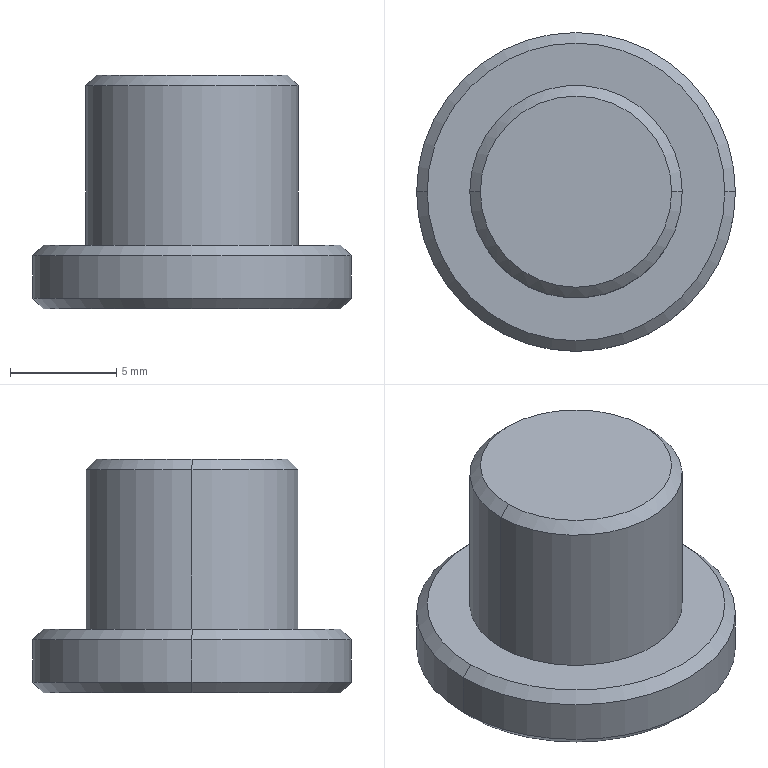Part | SolidWorks | features Chamfer 1, Revolution 1 | 1 solid | 13 faces | box 15 x 15 x 11 mm | volume 1143 mm3 | cone 6 | cylinder 4 | plane 3 | commonest cylinder face diameters 10 x2 15 x2
STEP:
#1=CARTESIAN_POINT('',(4.5,0.,0.));
#2=VERTEX_POINT('',#1);
#3=CARTESIAN_POINT('',(-4.5,0.,0.));
#4=VERTEX_POINT('',#3);
#5=CARTESIAN_POINT('',(0.,0.,0.));
#6=DIRECTION('',(0.,0.,1.));
#7=DIRECTION('',(-1.,0.,0.));
#8=AXIS2_PLACEMENT_3D('',#5,#6,#7);
#9=CIRCLE('',#8,4.5);
#10=EDGE_CURVE('',#2,#4,#9,.T.);
#11=ORIENTED_EDGE('',*,*,#10,.F.);
#12=CARTESIAN_POINT('',(5.,0.,-0.5));
#13=VERTEX_POINT('',#12);
#14=CARTESIAN_POINT('',(4.5,0.,0.));
#15=DIRECTION('',(0.7071,0.,-0.7071));
#16=VECTOR('',#15,1000.);
#17=LINE('',#14,#16);
#18=EDGE_CURVE('',#2,#13,#17,.T.);
#19=ORIENTED_EDGE('',*,*,#18,.T.);
#20=CARTESIAN_POINT('',(-5.,0.,-0.5));
#21=VERTEX_POINT('',#20);
#22=CARTESIAN_POINT('',(0.,0.,-0.5));
#23=DIRECTION('',(0.,0.,-1.));
#24=DIRECTION('',(-1.,0.,0.));
#25=AXIS2_PLACEMENT_3D('',#22,#23,#24);
#26=CIRCLE('',#25,5.);
#27=EDGE_CURVE('',#21,#13,#26,.T.);
#28=ORIENTED_EDGE('',*,*,#27,.F.);
#29=CARTESIAN_POINT('',(-4.5,0.,0.));
#30=DIRECTION('',(-0.7071,0.,-0.7071));
#31=VECTOR('',#30,1000.);
#32=LINE('',#29,#31);
#33=EDGE_CURVE('',#4,#21,#32,.T.);
#34=ORIENTED_EDGE('',*,*,#33,.F.);
#35=EDGE_LOOP('',(#11,#19,#28,#34));
#36=FACE_OUTER_BOUND('',#35,.T.);
#37=CARTESIAN_POINT('',(0.,0.,0.));
#38=DIRECTION('',(0.,0.,-1.));
#39=DIRECTION('',(-1.,0.,0.));
#40=AXIS2_PLACEMENT_3D('',#37,#38,#39);
#41=CONICAL_SURFACE('',#40,4.5,0.7854);
#42=ADVANCED_FACE('',(#36),#41,.T.);
#43=CARTESIAN_POINT('',(7.,0.,-8.));
#44=VERTEX_POINT('',#43);
#45=CARTESIAN_POINT('',(-7.,0.,-8.));
#46=VERTEX_POINT('',#45);
#47=CARTESIAN_POINT('',(0.,0.,-8.));
#48=DIRECTION('',(0.,0.,1.));
#49=DIRECTION('',(-1.,0.,0.));
#50=AXIS2_PLACEMENT_3D('',#47,#48,#49);
#51=CIRCLE('',#50,7.);
#52=EDGE_CURVE('',#44,#46,#51,.T.);
#53=ORIENTED_EDGE('',*,*,#52,.F.);
#54=CARTESIAN_POINT('',(7.5,0.,-8.5));
#55=VERTEX_POINT('',#54);
#56=CARTESIAN_POINT('',(7.,0.,-8.));
#57=DIRECTION('',(0.7071,0.,-0.7071));
#58=VECTOR('',#57,1000.);
#59=LINE('',#56,#58);
#60=EDGE_CURVE('',#44,#55,#59,.T.);
#61=ORIENTED_EDGE('',*,*,#60,.T.);
#62=CARTESIAN_POINT('',(-7.5,0.,-8.5));
#63=VERTEX_POINT('',#62);
#64=CARTESIAN_POINT('',(0.,0.,-8.5));
#65=DIRECTION('',(0.,0.,-1.));
#66=DIRECTION('',(-1.,0.,0.));
#67=AXIS2_PLACEMENT_3D('',#64,#65,#66);
#68=CIRCLE('',#67,7.5);
#69=EDGE_CURVE('',#63,#55,#68,.T.);
#70=ORIENTED_EDGE('',*,*,#69,.F.);
#71=CARTESIAN_POINT('',(-7.,0.,-8.));
#72=DIRECTION('',(-0.7071,0.,-0.7071));
#73=VECTOR('',#72,1000.);
#74=LINE('',#71,#73);
#75=EDGE_CURVE('',#46,#63,#74,.T.);
#76=ORIENTED_EDGE('',*,*,#75,.F.);
#77=EDGE_LOOP('',(#53,#61,#70,#76));
#78=FACE_OUTER_BOUND('',#77,.T.);
#79=CARTESIAN_POINT('',(0.,0.,-8.));
#80=DIRECTION('',(0.,0.,-1.));
#81=DIRECTION('',(-1.,0.,0.));
#82=AXIS2_PLACEMENT_3D('',#79,#80,#81);
#83=CONICAL_SURFACE('',#82,7.,0.7854);
#84=ADVANCED_FACE('',(#78),#83,.T.);
#85=CARTESIAN_POINT('',(-7.,0.,-11.));
#86=VERTEX_POINT('',#85);
#87=CARTESIAN_POINT('',(7.,0.,-11.));
#88=VERTEX_POINT('',#87);
#89=CARTESIAN_POINT('',(0.,0.,-11.));
#90=DIRECTION('',(0.,0.,-1.));
#91=DIRECTION('',(1.,0.,0.));
#92=AXIS2_PLACEMENT_3D('',#89,#90,#91);
#93=CIRCLE('',#92,7.);
#94=EDGE_CURVE('',#86,#88,#93,.T.);
#95=ORIENTED_EDGE('',*,*,#94,.F.);
#96=CARTESIAN_POINT('',(-7.5,0.,-10.5));
#97=VERTEX_POINT('',#96);
#98=CARTESIAN_POINT('',(-7.5,0.,-10.5));
#99=DIRECTION('',(-0.7071,0.,0.7071));
#100=VECTOR('',#99,1000.);
#101=LINE('',#98,#100);
#102=EDGE_CURVE('',#86,#97,#101,.T.);
#103=ORIENTED_EDGE('',*,*,#102,.T.);
#104=CARTESIAN_POINT('',(7.5,0.,-10.5));
#105=VERTEX_POINT('',#104);
#106=CARTESIAN_POINT('',(0.,0.,-10.5));
#107=DIRECTION('',(0.,0.,1.));
#108=DIRECTION('',(1.,0.,0.));
#109=AXIS2_PLACEMENT_3D('',#106,#107,#108);
#110=CIRCLE('',#109,7.5);
#111=EDGE_CURVE('',#105,#97,#110,.T.);
#112=ORIENTED_EDGE('',*,*,#111,.F.);
#113=CARTESIAN_POINT('',(7.5,0.,-10.5));
#114=DIRECTION('',(0.7071,0.,0.7071));
#115=VECTOR('',#114,1000.);
#116=LINE('',#113,#115);
#117=EDGE_CURVE('',#88,#105,#116,.T.);
#118=ORIENTED_EDGE('',*,*,#117,.F.);
#119=EDGE_LOOP('',(#95,#103,#112,#118));
#120=FACE_OUTER_BOUND('',#119,.T.);
#121=CARTESIAN_POINT('',(0.,0.,-10.5));
#122=DIRECTION('',(0.,0.,1.));
#123=DIRECTION('',(1.,0.,0.));
#124=AXIS2_PLACEMENT_3D('',#121,#122,#123);
#125=CONICAL_SURFACE('',#124,7.5,0.7854);
#126=ADVANCED_FACE('',(#120),#125,.T.);
#127=CARTESIAN_POINT('',(5.,0.,-8.));
#128=VERTEX_POINT('',#127);
#129=CARTESIAN_POINT('',(-5.,0.,-8.));
#130=VERTEX_POINT('',#129);
#131=CARTESIAN_POINT('',(0.,0.,-8.));
#132=DIRECTION('',(0.,0.,1.));
#133=DIRECTION('',(1.,0.,0.));
#134=AXIS2_PLACEMENT_3D('',#131,#132,#133);
#135=CIRCLE('',#134,5.);
#136=EDGE_CURVE('',#128,#130,#135,.T.);
#137=ORIENTED_EDGE('',*,*,#136,.T.);
#138=CARTESIAN_POINT('',(-5.,0.,0.));
#139=DIRECTION('',(0.,0.,1.));
#140=VECTOR('',#139,1000.);
#141=LINE('',#138,#140);
#142=EDGE_CURVE('',#130,#21,#141,.T.);
#143=ORIENTED_EDGE('',*,*,#142,.T.);
#144=ORIENTED_EDGE('',*,*,#27,.T.);
#145=CARTESIAN_POINT('',(5.,0.,0.));
#146=DIRECTION('',(0.,0.,1.));
#147=VECTOR('',#146,1000.);
#148=LINE('',#145,#147);
#149=EDGE_CURVE('',#128,#13,#148,.T.);
#150=ORIENTED_EDGE('',*,*,#149,.F.);
#151=EDGE_LOOP('',(#137,#143,#144,#150));
#152=FACE_OUTER_BOUND('',#151,.T.);
#153=CARTESIAN_POINT('',(0.,0.,0.));
#154=DIRECTION('',(0.,0.,1.));
#155=DIRECTION('',(1.,0.,0.));
#156=AXIS2_PLACEMENT_3D('',#153,#154,#155);
#157=CYLINDRICAL_SURFACE('',#156,5.);
#158=ADVANCED_FACE('',(#152),#157,.T.);
#159=ORIENTED_EDGE('',*,*,#111,.T.);
#160=CARTESIAN_POINT('',(-7.5,0.,0.));
#161=DIRECTION('',(0.,0.,1.));
#162=VECTOR('',#161,1000.);
#163=LINE('',#160,#162);
#164=EDGE_CURVE('',#97,#63,#163,.T.);
#165=ORIENTED_EDGE('',*,*,#164,.T.);
#166=ORIENTED_EDGE('',*,*,#69,.T.);
#167=CARTESIAN_POINT('',(7.5,0.,0.));
#168=DIRECTION('',(0.,0.,1.));
#169=VECTOR('',#168,1000.);
#170=LINE('',#167,#169);
#171=EDGE_CURVE('',#105,#55,#170,.T.);
#172=ORIENTED_EDGE('',*,*,#171,.F.);
#173=EDGE_LOOP('',(#159,#165,#166,#172));
#174=FACE_OUTER_BOUND('',#173,.T.);
#175=CARTESIAN_POINT('',(0.,0.,0.));
#176=DIRECTION('',(0.,0.,1.));
#177=DIRECTION('',(1.,0.,0.));
#178=AXIS2_PLACEMENT_3D('',#175,#176,#177);
#179=CYLINDRICAL_SURFACE('',#178,7.5);
#180=ADVANCED_FACE('',(#174),#179,.T.);
#181=CARTESIAN_POINT('',(0.,0.,-11.));
#182=DIRECTION('',(0.,0.,-1.));
#183=DIRECTION('',(1.,0.,0.));
#184=AXIS2_PLACEMENT_3D('',#181,#182,#183);
#185=CIRCLE('',#184,7.);
#186=EDGE_CURVE('',#88,#86,#185,.T.);
#187=ORIENTED_EDGE('',*,*,#186,.T.);
#188=ORIENTED_EDGE('',*,*,#94,.T.);
#189=EDGE_LOOP('',(#187,#188));
#190=FACE_OUTER_BOUND('',#189,.T.);
#191=CARTESIAN_POINT('',(0.,0.,-11.));
#192=DIRECTION('',(0.,0.,1.));
#193=DIRECTION('',(1.,0.,0.));
#194=AXIS2_PLACEMENT_3D('',#191,#192,#193);
#195=PLANE('',#194);
#196=ADVANCED_FACE('',(#190),#195,.F.);
#197=ORIENTED_EDGE('',*,*,#164,.F.);
#198=CARTESIAN_POINT('',(0.,0.,-10.5));
#199=DIRECTION('',(0.,0.,1.));
#200=DIRECTION('',(1.,0.,0.));
#201=AXIS2_PLACEMENT_3D('',#198,#199,#200);
#202=CIRCLE('',#201,7.5);
#203=EDGE_CURVE('',#97,#105,#202,.T.);
#204=ORIENTED_EDGE('',*,*,#203,.T.);
#205=ORIENTED_EDGE('',*,*,#171,.T.);
#206=CARTESIAN_POINT('',(0.,0.,-8.5));
#207=DIRECTION('',(0.,0.,-1.));
#208=DIRECTION('',(-1.,0.,0.));
#209=AXIS2_PLACEMENT_3D('',#206,#207,#208);
#210=CIRCLE('',#209,7.5);
#211=EDGE_CURVE('',#55,#63,#210,.T.);
#212=ORIENTED_EDGE('',*,*,#211,.T.);
#213=EDGE_LOOP('',(#197,#204,#205,#212));
#214=FACE_OUTER_BOUND('',#213,.T.);
#215=CARTESIAN_POINT('',(0.,0.,0.));
#216=DIRECTION('',(0.,0.,1.));
#217=DIRECTION('',(1.,0.,0.));
#218=AXIS2_PLACEMENT_3D('',#215,#216,#217);
#219=CYLINDRICAL_SURFACE('',#218,7.5);
#220=ADVANCED_FACE('',(#214),#219,.T.);
#221=CARTESIAN_POINT('',(0.,0.,-8.));
#222=DIRECTION('',(0.,0.,1.));
#223=DIRECTION('',(-1.,0.,0.));
#224=AXIS2_PLACEMENT_3D('',#221,#222,#223);
#225=CIRCLE('',#224,7.);
#226=EDGE_CURVE('',#46,#44,#225,.T.);
#227=ORIENTED_EDGE('',*,*,#226,.T.);
#228=ORIENTED_EDGE('',*,*,#52,.T.);
#229=EDGE_LOOP('',(#227,#228));
#230=FACE_OUTER_BOUND('',#229,.T.);
#231=ORIENTED_EDGE('',*,*,#136,.F.);
#232=CARTESIAN_POINT('',(0.,0.,-8.));
#233=DIRECTION('',(0.,0.,1.));
#234=DIRECTION('',(1.,0.,0.));
#235=AXIS2_PLACEMENT_3D('',#232,#233,#234);
#236=CIRCLE('',#235,5.);
#237=EDGE_CURVE('',#130,#128,#236,.T.);
#238=ORIENTED_EDGE('',*,*,#237,.F.);
#239=EDGE_LOOP('',(#231,#238));
#240=FACE_BOUND('',#239,.T.);
#241=CARTESIAN_POINT('',(0.,7.5,-8.));
#242=DIRECTION('',(0.,0.,-1.));
#243=DIRECTION('',(-1.,0.,0.));
#244=AXIS2_PLACEMENT_3D('',#241,#242,#243);
#245=PLANE('',#244);
#246=ADVANCED_FACE('',(#230,#240),#245,.F.);
#247=ORIENTED_EDGE('',*,*,#142,.F.);
#248=ORIENTED_EDGE('',*,*,#237,.T.);
#249=ORIENTED_EDGE('',*,*,#149,.T.);
#250=CARTESIAN_POINT('',(0.,0.,-0.5));
#251=DIRECTION('',(0.,0.,-1.));
#252=DIRECTION('',(-1.,0.,0.));
#253=AXIS2_PLACEMENT_3D('',#250,#251,#252);
#254=CIRCLE('',#253,5.);
#255=EDGE_CURVE('',#13,#21,#254,.T.);
#256=ORIENTED_EDGE('',*,*,#255,.T.);
#257=EDGE_LOOP('',(#247,#248,#249,#256));
#258=FACE_OUTER_BOUND('',#257,.T.);
#259=CARTESIAN_POINT('',(0.,0.,0.));
#260=DIRECTION('',(0.,0.,1.));
#261=DIRECTION('',(1.,0.,0.));
#262=AXIS2_PLACEMENT_3D('',#259,#260,#261);
#263=CYLINDRICAL_SURFACE('',#262,5.);
#264=ADVANCED_FACE('',(#258),#263,.T.);
#265=CARTESIAN_POINT('',(0.,0.,0.));
#266=DIRECTION('',(0.,0.,1.));
#267=DIRECTION('',(-1.,0.,0.));
#268=AXIS2_PLACEMENT_3D('',#265,#266,#267);
#269=CIRCLE('',#268,4.5);
#270=EDGE_CURVE('',#4,#2,#269,.T.);
#271=ORIENTED_EDGE('',*,*,#270,.T.);
#272=ORIENTED_EDGE('',*,*,#10,.T.);
#273=EDGE_LOOP('',(#271,#272));
#274=FACE_OUTER_BOUND('',#273,.T.);
#275=CARTESIAN_POINT('',(0.,5.,0.));
#276=DIRECTION('',(0.,0.,-1.));
#277=DIRECTION('',(-1.,0.,0.));
#278=AXIS2_PLACEMENT_3D('',#275,#276,#277);
#279=PLANE('',#278);
#280=ADVANCED_FACE('',(#274),#279,.F.);
#281=ORIENTED_EDGE('',*,*,#102,.F.);
#282=ORIENTED_EDGE('',*,*,#186,.F.);
#283=ORIENTED_EDGE('',*,*,#117,.T.);
#284=ORIENTED_EDGE('',*,*,#203,.F.);
#285=EDGE_LOOP('',(#281,#282,#283,#284));
#286=FACE_OUTER_BOUND('',#285,.T.);
#287=CARTESIAN_POINT('',(0.,0.,-10.5));
#288=DIRECTION('',(0.,0.,1.));
#289=DIRECTION('',(1.,0.,0.));
#290=AXIS2_PLACEMENT_3D('',#287,#288,#289);
#291=CONICAL_SURFACE('',#290,7.5,0.7854);
#292=ADVANCED_FACE('',(#286),#291,.T.);
#293=ORIENTED_EDGE('',*,*,#60,.F.);
#294=ORIENTED_EDGE('',*,*,#226,.F.);
#295=ORIENTED_EDGE('',*,*,#75,.T.);
#296=ORIENTED_EDGE('',*,*,#211,.F.);
#297=EDGE_LOOP('',(#293,#294,#295,#296));
#298=FACE_OUTER_BOUND('',#297,.T.);
#299=CARTESIAN_POINT('',(0.,0.,-8.));
#300=DIRECTION('',(0.,0.,-1.));
#301=DIRECTION('',(-1.,0.,0.));
#302=AXIS2_PLACEMENT_3D('',#299,#300,#301);
#303=CONICAL_SURFACE('',#302,7.,0.7854);
#304=ADVANCED_FACE('',(#298),#303,.T.);
#305=ORIENTED_EDGE('',*,*,#18,.F.);
#306=ORIENTED_EDGE('',*,*,#270,.F.);
#307=ORIENTED_EDGE('',*,*,#33,.T.);
#308=ORIENTED_EDGE('',*,*,#255,.F.);
#309=EDGE_LOOP('',(#305,#306,#307,#308));
#310=FACE_OUTER_BOUND('',#309,.T.);
#311=CARTESIAN_POINT('',(0.,0.,0.));
#312=DIRECTION('',(0.,0.,-1.));
#313=DIRECTION('',(-1.,0.,0.));
#314=AXIS2_PLACEMENT_3D('',#311,#312,#313);
#315=CONICAL_SURFACE('',#314,4.5,0.7854);
#316=ADVANCED_FACE('',(#310),#315,.T.);
#317=CLOSED_SHELL('',(#42,#84,#126,#158,#180,#196,#220,#246,#264,#280,#292,#304,#316));
#318=MANIFOLD_SOLID_BREP('',#317);
#319=CARTESIAN_POINT('',(0.,0.,0.));
#320=DIRECTION('',(0.,0.,1.));
#321=DIRECTION('',(1.,0.,0.));
#322=AXIS2_PLACEMENT_3D('',#319,#320,#321);
#323=(LENGTH_UNIT()NAMED_UNIT(*)SI_UNIT(.MILLI.,.METRE.));
#324=UNCERTAINTY_MEASURE_WITH_UNIT(LENGTH_MEASURE(0.00001),#323,'','');
#325=(NAMED_UNIT(*)PLANE_ANGLE_UNIT()SI_UNIT($,.RADIAN.));
#326=(NAMED_UNIT(*)SI_UNIT($,.STERADIAN.)SOLID_ANGLE_UNIT());
#327=(GEOMETRIC_REPRESENTATION_CONTEXT(3)GLOBAL_UNCERTAINTY_ASSIGNED_CONTEXT((#324))GLOBAL_UNIT_ASSIGNED_CONTEXT((#323,#325,#326))REPRESENTATION_CONTEXT('',''));
#328=ADVANCED_BREP_SHAPE_REPRESENTATION('',(#318,#322),#327);